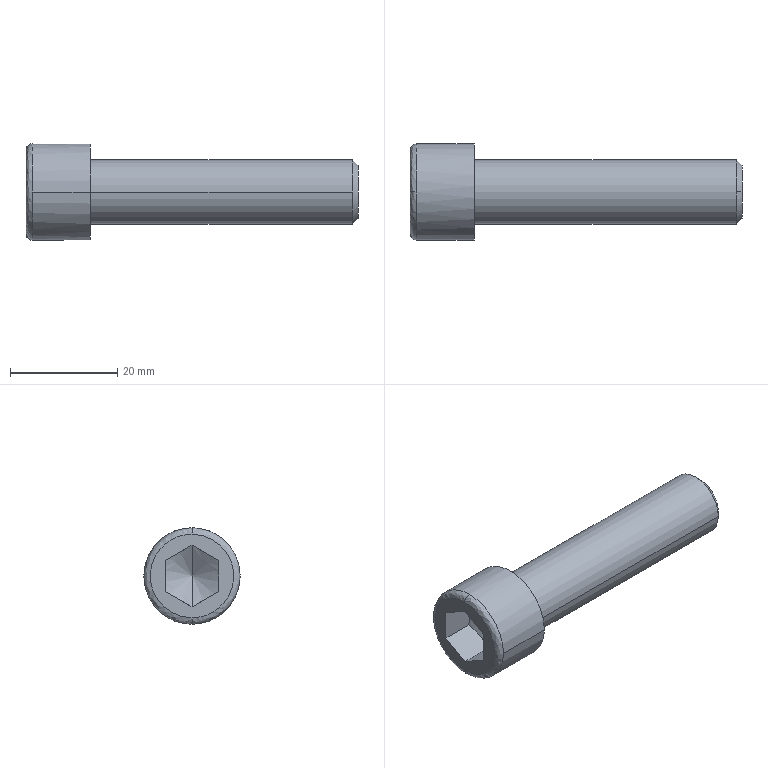Part | SolidWorks | features BaseBody 1 | 1 solid | 21 faces | box 62 x 18 x 18 mm | volume 8038 mm3 | plane 9 | spline 4 | cylinder 4 | cone 4 | commonest cylinder face diameters 12 x2 18 x2
STEP:
#1=CARTESIAN_POINT('',(0.,0.,6.1));
#2=VERTEX_POINT('',#1);
#3=CARTESIAN_POINT('',(0.,0.,-6.1));
#4=VERTEX_POINT('',#3);
#5=CARTESIAN_POINT('',(0.,0.,6.1));
#6=CARTESIAN_POINT('',(0.,0.1864,6.1));
#7=CARTESIAN_POINT('',(0.,0.4649,6.087));
#8=CARTESIAN_POINT('',(0.,0.788,6.05));
#9=CARTESIAN_POINT('',(0.,0.9492,6.026));
#10=CARTESIAN_POINT('',(0.,1.018,6.014));
#11=CARTESIAN_POINT('',(0.,1.064,6.007));
#12=CARTESIAN_POINT('',(0.,1.086,6.003));
#13=CARTESIAN_POINT('',(0.,1.304,5.962));
#14=CARTESIAN_POINT('',(0.,1.592,5.894));
#15=CARTESIAN_POINT('',(0.,1.921,5.791));
#16=CARTESIAN_POINT('',(0.,2.06,5.742));
#17=CARTESIAN_POINT('',(0.,2.153,5.708));
#18=CARTESIAN_POINT('',(0.,2.198,5.691));
#19=CARTESIAN_POINT('',(0.,2.437,5.596));
#20=CARTESIAN_POINT('',(0.,2.717,5.468));
#21=CARTESIAN_POINT('',(0.,2.987,5.32));
#22=CARTESIAN_POINT('',(0.,3.164,5.216));
#23=CARTESIAN_POINT('',(0.,3.25,5.163));
#24=CARTESIAN_POINT('',(0.,3.69,4.875));
#25=CARTESIAN_POINT('',(0.,4.016,4.611));
#26=CARTESIAN_POINT('',(0.,4.462,4.165));
#27=CARTESIAN_POINT('',(0.,4.673,3.931));
#28=CARTESIAN_POINT('',(0.,4.897,3.641));
#29=CARTESIAN_POINT('',(0.,4.988,3.512));
#30=CARTESIAN_POINT('',(0.,5.047,3.426));
#31=CARTESIAN_POINT('',(0.,5.077,3.381));
#32=CARTESIAN_POINT('',(0.,5.218,3.166));
#33=CARTESIAN_POINT('',(0.,5.374,2.9));
#34=CARTESIAN_POINT('',(0.,5.531,2.577));
#35=CARTESIAN_POINT('',(0.,5.593,2.436));
#36=CARTESIAN_POINT('',(0.,5.633,2.341));
#37=CARTESIAN_POINT('',(0.,5.654,2.291));
#38=CARTESIAN_POINT('',(0.,5.744,2.062));
#39=CARTESIAN_POINT('',(0.,5.84,1.782));
#40=CARTESIAN_POINT('',(0.,5.927,1.448));
#41=CARTESIAN_POINT('',(0.,5.965,1.28));
#42=CARTESIAN_POINT('',(0.,5.979,1.207));
#43=CARTESIAN_POINT('',(0.,5.989,1.159));
#44=CARTESIAN_POINT('',(0.,5.994,1.133));
#45=CARTESIAN_POINT('',(0.,6.066,0.7429));
#46=CARTESIAN_POINT('',(0.,6.1,0.3729));
#47=CARTESIAN_POINT('',(0.,6.1,-0.1865));
#48=CARTESIAN_POINT('',(0.,6.091,-0.3725));
#49=CARTESIAN_POINT('',(0.,6.066,-0.65));
#50=CARTESIAN_POINT('',(0.,6.05,-0.7884));
#51=CARTESIAN_POINT('',(0.,6.026,-0.9494));
#52=CARTESIAN_POINT('',(0.,6.014,-1.018));
#53=CARTESIAN_POINT('',(0.,6.007,-1.064));
#54=CARTESIAN_POINT('',(0.,6.003,-1.086));
#55=CARTESIAN_POINT('',(0.,5.962,-1.304));
#56=CARTESIAN_POINT('',(0.,5.894,-1.592));
#57=CARTESIAN_POINT('',(0.,5.791,-1.921));
#58=CARTESIAN_POINT('',(0.,5.742,-2.06));
#59=CARTESIAN_POINT('',(0.,5.708,-2.153));
#60=CARTESIAN_POINT('',(0.,5.691,-2.198));
#61=CARTESIAN_POINT('',(0.,5.596,-2.437));
#62=CARTESIAN_POINT('',(0.,5.468,-2.717));
#63=CARTESIAN_POINT('',(0.,5.32,-2.987));
#64=CARTESIAN_POINT('',(0.,5.216,-3.164));
#65=CARTESIAN_POINT('',(0.,5.163,-3.25));
#66=CARTESIAN_POINT('',(0.,4.875,-3.69));
#67=CARTESIAN_POINT('',(0.,4.611,-4.016));
#68=CARTESIAN_POINT('',(0.,4.165,-4.462));
#69=CARTESIAN_POINT('',(0.,3.931,-4.673));
#70=CARTESIAN_POINT('',(0.,3.641,-4.897));
#71=CARTESIAN_POINT('',(0.,3.512,-4.988));
#72=CARTESIAN_POINT('',(0.,3.426,-5.047));
#73=CARTESIAN_POINT('',(0.,3.381,-5.077));
#74=CARTESIAN_POINT('',(0.,3.166,-5.218));
#75=CARTESIAN_POINT('',(0.,2.9,-5.374));
#76=CARTESIAN_POINT('',(0.,2.577,-5.531));
#77=CARTESIAN_POINT('',(0.,2.436,-5.593));
#78=CARTESIAN_POINT('',(0.,2.341,-5.633));
#79=CARTESIAN_POINT('',(0.,2.291,-5.654));
#80=CARTESIAN_POINT('',(0.,2.062,-5.744));
#81=CARTESIAN_POINT('',(0.,1.782,-5.84));
#82=CARTESIAN_POINT('',(0.,1.448,-5.927));
#83=CARTESIAN_POINT('',(0.,1.28,-5.965));
#84=CARTESIAN_POINT('',(0.,1.207,-5.979));
#85=CARTESIAN_POINT('',(0.,1.159,-5.989));
#86=CARTESIAN_POINT('',(0.,1.133,-5.994));
#87=CARTESIAN_POINT('',(0.,0.7435,-6.066));
#88=CARTESIAN_POINT('',(0.,0.3728,-6.1));
#89=CARTESIAN_POINT('',(0.,0.,-6.1));
#90=B_SPLINE_CURVE_WITH_KNOTS('',3,(#5,#6,#7,#8,#9,#10,#11,#12,#13,#14,#15,#16,#17,#18,#19,#20,#21,#22,#23,#24,#25,#26,#27,#28,#29,#30,#31,#32,#33,#34,#35,#36,#37,#38,#39,#40,#41,#42,#43,#44,#45,#46,#47,#48,#49,#50,#51,#52,#53,#54,#55,#56,#57,#58,#59,#60,#61,#62,#63,#64,#65,#66,#67,#68,#69,#70,#71,#72,#73,#74,#75,#76,#77,#78,#79,#80,#81,#82,#83,#84,#85,#86,#87,#88,#89),.UNSPECIFIED.,.F.,.F.,(4,1,1,1,2,2,1,1,2,2,1,2,2,2,1,1,2,2,1,1,2,2,1,1,1,2,2,2,2,1,1,2,2,1,1,2,2,1,2,2,2,1,1,2,2,1,1,2,2,1,1,1,2,2,4),(0.75,0.7656,0.7734,0.7773,0.7793,0.7812,0.7969,0.8047,0.8086,0.8125,0.8281,0.8359,0.8437,0.875,0.8906,0.8984,0.9023,0.9063,0.9219,0.9297,0.9336,0.9375,0.9531,0.9609,0.9648,0.9668,0.9688,1.,1.016,1.023,1.027,1.029,1.031,1.047,1.055,1.059,1.063,1.078,1.086,1.094,1.125,1.141,1.148,1.152,1.156,1.172,1.18,1.184,1.188,1.203,1.211,1.215,1.217,1.219,1.25),.UNSPECIFIED.);
#91=EDGE_CURVE('',#2,#4,#90,.T.);
#92=ORIENTED_EDGE('',*,*,#91,.F.);
#93=CARTESIAN_POINT('',(0.1,0.,6.));
#94=VERTEX_POINT('',#93);
#95=CARTESIAN_POINT('',(0.1,0.,6.1));
#96=DIRECTION('',(0.,-1.,0.));
#97=DIRECTION('',(0.,0.,1.));
#98=AXIS2_PLACEMENT_3D('',#95,#96,#97);
#99=CIRCLE('',#98,0.1);
#100=EDGE_CURVE('',#2,#94,#99,.T.);
#101=ORIENTED_EDGE('',*,*,#100,.T.);
#102=CARTESIAN_POINT('',(0.1,6.,0.));
#103=VERTEX_POINT('',#102);
#104=CARTESIAN_POINT('',(0.1,0.,0.));
#105=DIRECTION('',(1.,0.,0.));
#106=DIRECTION('',(0.,1.,0.));
#107=AXIS2_PLACEMENT_3D('',#104,#105,#106);
#108=CIRCLE('',#107,6.);
#109=EDGE_CURVE('',#103,#94,#108,.T.);
#110=ORIENTED_EDGE('',*,*,#109,.F.);
#111=CARTESIAN_POINT('',(0.1,0.,-6.));
#112=VERTEX_POINT('',#111);
#113=CARTESIAN_POINT('',(0.1,0.,0.));
#114=DIRECTION('',(1.,0.,0.));
#115=DIRECTION('',(0.,1.,0.));
#116=AXIS2_PLACEMENT_3D('',#113,#114,#115);
#117=CIRCLE('',#116,6.);
#118=EDGE_CURVE('',#112,#103,#117,.T.);
#119=ORIENTED_EDGE('',*,*,#118,.F.);
#120=CARTESIAN_POINT('',(0.1,0.,-6.1));
#121=DIRECTION('',(0.,1.,0.));
#122=DIRECTION('',(0.,0.,-1.));
#123=AXIS2_PLACEMENT_3D('',#120,#121,#122);
#124=CIRCLE('',#123,0.1);
#125=EDGE_CURVE('',#4,#112,#124,.T.);
#126=ORIENTED_EDGE('',*,*,#125,.F.);
#127=EDGE_LOOP('',(#92,#101,#110,#119,#126));
#128=FACE_OUTER_BOUND('',#127,.T.);
#129=CARTESIAN_POINT('',(0.,0.,-6.1));
#130=CARTESIAN_POINT('',(0.,12.2,-6.1));
#131=CARTESIAN_POINT('',(0.,12.2,6.1));
#132=CARTESIAN_POINT('',(0.,0.,6.1));
#133=CARTESIAN_POINT('',(0.,0.,-6.041));
#134=CARTESIAN_POINT('',(0.,12.083,-6.041));
#135=CARTESIAN_POINT('',(0.,12.083,6.041));
#136=CARTESIAN_POINT('',(0.,0.,6.041));
#137=CARTESIAN_POINT('',(0.04142,0.,-6.));
#138=CARTESIAN_POINT('',(0.04142,12.,-6.));
#139=CARTESIAN_POINT('',(0.04142,12.,6.));
#140=CARTESIAN_POINT('',(0.04142,0.,6.));
#141=CARTESIAN_POINT('',(0.1,0.,-6.));
#142=CARTESIAN_POINT('',(0.1,12.,-6.));
#143=CARTESIAN_POINT('',(0.1,12.,6.));
#144=CARTESIAN_POINT('',(0.1,0.,6.));
#145=(BOUNDED_SURFACE()B_SPLINE_SURFACE(3,3,((#129,#130,#131,#132),(#133,#134,#135,#136),(#137,#138,#139,#140),(#141,#142,#143,#144)),.UNSPECIFIED.,.F.,.F.,.T.)B_SPLINE_SURFACE_WITH_KNOTS((4,4),(4,4),(0.,1.),(0.,1.),.UNSPECIFIED.)GEOMETRIC_REPRESENTATION_ITEM()RATIONAL_B_SPLINE_SURFACE(((1.,0.3333,0.3333,1.),(0.8047,0.2682,0.2682,0.8047),(0.8047,0.2682,0.2682,0.8047),(1.,0.3333,0.3333,1.)))REPRESENTATION_ITEM('')SURFACE());
#146=ADVANCED_FACE('',(#128),#145,.F.);
#147=CARTESIAN_POINT('',(-10.8,0.,9.));
#148=VERTEX_POINT('',#147);
#149=CARTESIAN_POINT('',(-10.8,-9.,0.));
#150=VERTEX_POINT('',#149);
#151=CARTESIAN_POINT('',(-10.8,0.,0.));
#152=DIRECTION('',(1.,0.,0.));
#153=DIRECTION('',(0.,1.,0.));
#154=AXIS2_PLACEMENT_3D('',#151,#152,#153);
#155=CIRCLE('',#154,9.);
#156=EDGE_CURVE('',#148,#150,#155,.T.);
#157=ORIENTED_EDGE('',*,*,#156,.F.);
#158=CARTESIAN_POINT('',(-12.,0.,7.8));
#159=VERTEX_POINT('',#158);
#160=CARTESIAN_POINT('',(-10.8,0.,7.8));
#161=DIRECTION('',(0.,-1.,0.));
#162=DIRECTION('',(0.,0.,1.));
#163=AXIS2_PLACEMENT_3D('',#160,#161,#162);
#164=CIRCLE('',#163,1.2);
#165=EDGE_CURVE('',#148,#159,#164,.T.);
#166=ORIENTED_EDGE('',*,*,#165,.T.);
#167=CARTESIAN_POINT('',(-12.,0.,-7.8));
#168=VERTEX_POINT('',#167);
#169=CARTESIAN_POINT('',(-12.,0.,7.8));
#170=CARTESIAN_POINT('',(-12.,-15.6,7.8));
#171=CARTESIAN_POINT('',(-12.,-15.6,-7.8));
#172=CARTESIAN_POINT('',(-12.,0.,-7.8));
#173=(BOUNDED_CURVE()B_SPLINE_CURVE(3,(#169,#170,#171,#172),.UNSPECIFIED.,.F.,.T.)B_SPLINE_CURVE_WITH_KNOTS((4,4),(0.25,0.75),.UNSPECIFIED.)CURVE()GEOMETRIC_REPRESENTATION_ITEM()RATIONAL_B_SPLINE_CURVE((1.,0.3333,0.3333,1.))REPRESENTATION_ITEM(''));
#174=EDGE_CURVE('',#159,#168,#173,.T.);
#175=ORIENTED_EDGE('',*,*,#174,.T.);
#176=CARTESIAN_POINT('',(-10.8,0.,-9.));
#177=VERTEX_POINT('',#176);
#178=CARTESIAN_POINT('',(-10.8,0.,-7.8));
#179=DIRECTION('',(0.,1.,0.));
#180=DIRECTION('',(0.,0.,-1.));
#181=AXIS2_PLACEMENT_3D('',#178,#179,#180);
#182=CIRCLE('',#181,1.2);
#183=EDGE_CURVE('',#177,#168,#182,.T.);
#184=ORIENTED_EDGE('',*,*,#183,.F.);
#185=CARTESIAN_POINT('',(-10.8,0.,0.));
#186=DIRECTION('',(1.,0.,0.));
#187=DIRECTION('',(0.,1.,0.));
#188=AXIS2_PLACEMENT_3D('',#185,#186,#187);
#189=CIRCLE('',#188,9.);
#190=EDGE_CURVE('',#150,#177,#189,.T.);
#191=ORIENTED_EDGE('',*,*,#190,.F.);
#192=EDGE_LOOP('',(#157,#166,#175,#184,#191));
#193=FACE_OUTER_BOUND('',#192,.T.);
#194=CARTESIAN_POINT('',(-10.8,0.,9.));
#195=CARTESIAN_POINT('',(-10.8,-18.,9.));
#196=CARTESIAN_POINT('',(-10.8,-18.,-9.));
#197=CARTESIAN_POINT('',(-10.8,0.,-9.));
#198=CARTESIAN_POINT('',(-11.503,0.,9.));
#199=CARTESIAN_POINT('',(-11.503,-18.,9.));
#200=CARTESIAN_POINT('',(-11.503,-18.,-9.));
#201=CARTESIAN_POINT('',(-11.503,0.,-9.));
#202=CARTESIAN_POINT('',(-12.,0.,8.503));
#203=CARTESIAN_POINT('',(-12.,-17.006,8.503));
#204=CARTESIAN_POINT('',(-12.,-17.006,-8.503));
#205=CARTESIAN_POINT('',(-12.,0.,-8.503));
#206=CARTESIAN_POINT('',(-12.,0.,7.8));
#207=CARTESIAN_POINT('',(-12.,-15.6,7.8));
#208=CARTESIAN_POINT('',(-12.,-15.6,-7.8));
#209=CARTESIAN_POINT('',(-12.,0.,-7.8));
#210=(BOUNDED_SURFACE()B_SPLINE_SURFACE(3,3,((#194,#195,#196,#197),(#198,#199,#200,#201),(#202,#203,#204,#205),(#206,#207,#208,#209)),.UNSPECIFIED.,.F.,.F.,.T.)B_SPLINE_SURFACE_WITH_KNOTS((4,4),(4,4),(0.,1.),(0.,1.),.UNSPECIFIED.)GEOMETRIC_REPRESENTATION_ITEM()RATIONAL_B_SPLINE_SURFACE(((1.,0.3333,0.3333,1.),(0.8047,0.2682,0.2682,0.8047),(0.8047,0.2682,0.2682,0.8047),(1.,0.3333,0.3333,1.)))REPRESENTATION_ITEM('')SURFACE());
#211=ADVANCED_FACE('',(#193),#210,.T.);
#212=ORIENTED_EDGE('',*,*,#109,.T.);
#213=CARTESIAN_POINT('',(0.1,-6.,0.));
#214=VERTEX_POINT('',#213);
#215=CARTESIAN_POINT('',(0.1,0.,0.));
#216=DIRECTION('',(1.,0.,0.));
#217=DIRECTION('',(0.,1.,0.));
#218=AXIS2_PLACEMENT_3D('',#215,#216,#217);
#219=CIRCLE('',#218,6.);
#220=EDGE_CURVE('',#94,#214,#219,.T.);
#221=ORIENTED_EDGE('',*,*,#220,.T.);
#222=CARTESIAN_POINT('',(48.926,-6.,0.));
#223=VERTEX_POINT('',#222);
#224=CARTESIAN_POINT('',(35.,-6.,0.));
#225=DIRECTION('',(1.,0.,0.));
#226=VECTOR('',#225,1000.);
#227=LINE('',#224,#226);
#228=EDGE_CURVE('',#214,#223,#227,.T.);
#229=ORIENTED_EDGE('',*,*,#228,.T.);
#230=CARTESIAN_POINT('',(48.926,0.,6.));
#231=VERTEX_POINT('',#230);
#232=CARTESIAN_POINT('',(48.926,0.,0.));
#233=DIRECTION('',(-1.,0.,0.));
#234=DIRECTION('',(0.,1.,0.));
#235=AXIS2_PLACEMENT_3D('',#232,#233,#234);
#236=CIRCLE('',#235,6.);
#237=EDGE_CURVE('',#223,#231,#236,.T.);
#238=ORIENTED_EDGE('',*,*,#237,.T.);
#239=CARTESIAN_POINT('',(48.926,6.,0.));
#240=VERTEX_POINT('',#239);
#241=CARTESIAN_POINT('',(48.926,0.,0.));
#242=DIRECTION('',(-1.,0.,0.));
#243=DIRECTION('',(0.,1.,0.));
#244=AXIS2_PLACEMENT_3D('',#241,#242,#243);
#245=CIRCLE('',#244,6.);
#246=EDGE_CURVE('',#231,#240,#245,.T.);
#247=ORIENTED_EDGE('',*,*,#246,.T.);
#248=CARTESIAN_POINT('',(35.,6.,0.));
#249=DIRECTION('',(1.,0.,0.));
#250=VECTOR('',#249,1000.);
#251=LINE('',#248,#250);
#252=EDGE_CURVE('',#103,#240,#251,.T.);
#253=ORIENTED_EDGE('',*,*,#252,.F.);
#254=EDGE_LOOP('',(#212,#221,#229,#238,#247,#253));
#255=FACE_OUTER_BOUND('',#254,.T.);
#256=CARTESIAN_POINT('',(35.,0.,0.));
#257=DIRECTION('',(1.,0.,0.));
#258=DIRECTION('',(0.,1.,0.));
#259=AXIS2_PLACEMENT_3D('',#256,#257,#258);
#260=CYLINDRICAL_SURFACE('',#259,6.);
#261=ADVANCED_FACE('',(#255),#260,.T.);
#262=CARTESIAN_POINT('',(50.,0.,4.926));
#263=VERTEX_POINT('',#262);
#264=CARTESIAN_POINT('',(50.,0.,-4.926));
#265=VERTEX_POINT('',#264);
#266=CARTESIAN_POINT('',(50.,0.,0.));
#267=DIRECTION('',(-1.,0.,0.));
#268=DIRECTION('',(0.,0.,1.));
#269=AXIS2_PLACEMENT_3D('',#266,#267,#268);
#270=CIRCLE('',#269,4.926);
#271=EDGE_CURVE('',#263,#265,#270,.T.);
#272=ORIENTED_EDGE('',*,*,#271,.T.);
#273=CARTESIAN_POINT('',(48.926,0.,-6.));
#274=VERTEX_POINT('',#273);
#275=CARTESIAN_POINT('',(48.926,0.,-6.));
#276=DIRECTION('',(-0.7071,0.,-0.7071));
#277=VECTOR('',#276,1000.);
#278=LINE('',#275,#277);
#279=EDGE_CURVE('',#265,#274,#278,.T.);
#280=ORIENTED_EDGE('',*,*,#279,.T.);
#281=CARTESIAN_POINT('',(48.926,0.,0.));
#282=DIRECTION('',(-1.,0.,0.));
#283=DIRECTION('',(0.,1.,0.));
#284=AXIS2_PLACEMENT_3D('',#281,#282,#283);
#285=CIRCLE('',#284,6.);
#286=EDGE_CURVE('',#240,#274,#285,.T.);
#287=ORIENTED_EDGE('',*,*,#286,.F.);
#288=ORIENTED_EDGE('',*,*,#246,.F.);
#289=CARTESIAN_POINT('',(48.926,0.,6.));
#290=DIRECTION('',(-0.7071,0.,0.7071));
#291=VECTOR('',#290,1000.);
#292=LINE('',#289,#291);
#293=EDGE_CURVE('',#263,#231,#292,.T.);
#294=ORIENTED_EDGE('',*,*,#293,.F.);
#295=EDGE_LOOP('',(#272,#280,#287,#288,#294));
#296=FACE_OUTER_BOUND('',#295,.T.);
#297=CARTESIAN_POINT('',(48.926,0.,0.));
#298=DIRECTION('',(-1.,0.,0.));
#299=DIRECTION('',(0.,0.,1.));
#300=AXIS2_PLACEMENT_3D('',#297,#298,#299);
#301=CONICAL_SURFACE('',#300,6.,0.7854);
#302=ADVANCED_FACE('',(#296),#301,.T.);
#303=CARTESIAN_POINT('',(-10.8,9.,0.));
#304=VERTEX_POINT('',#303);
#305=CARTESIAN_POINT('',(-10.8,0.,0.));
#306=DIRECTION('',(1.,0.,0.));
#307=DIRECTION('',(0.,1.,0.));
#308=AXIS2_PLACEMENT_3D('',#305,#306,#307);
#309=CIRCLE('',#308,9.);
#310=EDGE_CURVE('',#304,#148,#309,.T.);
#311=ORIENTED_EDGE('',*,*,#310,.T.);
#312=ORIENTED_EDGE('',*,*,#156,.T.);
#313=CARTESIAN_POINT('',(0.,-9.,0.));
#314=VERTEX_POINT('',#313);
#315=CARTESIAN_POINT('',(-6.,-9.,0.));
#316=DIRECTION('',(1.,0.,0.));
#317=VECTOR('',#316,1000.);
#318=LINE('',#315,#317);
#319=EDGE_CURVE('',#150,#314,#318,.T.);
#320=ORIENTED_EDGE('',*,*,#319,.T.);
#321=CARTESIAN_POINT('',(0.,9.,0.));
#322=VERTEX_POINT('',#321);
#323=CARTESIAN_POINT('',(0.,0.,0.));
#324=DIRECTION('',(1.,0.,0.));
#325=DIRECTION('',(0.,1.,0.));
#326=AXIS2_PLACEMENT_3D('',#323,#324,#325);
#327=CIRCLE('',#326,9.);
#328=EDGE_CURVE('',#322,#314,#327,.T.);
#329=ORIENTED_EDGE('',*,*,#328,.F.);
#330=CARTESIAN_POINT('',(-6.,9.,0.));
#331=DIRECTION('',(1.,0.,0.));
#332=VECTOR('',#331,1000.);
#333=LINE('',#330,#332);
#334=EDGE_CURVE('',#304,#322,#333,.T.);
#335=ORIENTED_EDGE('',*,*,#334,.F.);
#336=EDGE_LOOP('',(#311,#312,#320,#329,#335));
#337=FACE_OUTER_BOUND('',#336,.T.);
#338=CARTESIAN_POINT('',(-6.,0.,0.));
#339=DIRECTION('',(1.,0.,0.));
#340=DIRECTION('',(0.,1.,0.));
#341=AXIS2_PLACEMENT_3D('',#338,#339,#340);
#342=CYLINDRICAL_SURFACE('',#341,9.);
#343=ADVANCED_FACE('',(#337),#342,.T.);
#344=CARTESIAN_POINT('',(-2.667,0.,0.));
#345=VERTEX_POINT('',#344);
#346=CARTESIAN_POINT('',(-6.,0.,5.774));
#347=VERTEX_POINT('',#346);
#348=CARTESIAN_POINT('',(-6.02,0.,5.808));
#349=DIRECTION('',(-0.5,0.,0.866));
#350=VECTOR('',#349,1000.);
#351=LINE('',#348,#350);
#352=EDGE_CURVE('',#345,#347,#351,.T.);
#353=ORIENTED_EDGE('',*,*,#352,.F.);
#354=CARTESIAN_POINT('',(-6.,0.,-5.774));
#355=VERTEX_POINT('',#354);
#356=CARTESIAN_POINT('',(-6.02,0.,-5.808));
#357=DIRECTION('',(-0.5,0.,-0.866));
#358=VECTOR('',#357,1000.);
#359=LINE('',#356,#358);
#360=EDGE_CURVE('',#345,#355,#359,.T.);
#361=ORIENTED_EDGE('',*,*,#360,.T.);
#362=CARTESIAN_POINT('',(-6.,-5.,-2.887));
#363=VERTEX_POINT('',#362);
#364=CARTESIAN_POINT('',(-6.,0.,-5.774));
#365=CARTESIAN_POINT('',(-5.728,-0.8164,-5.302));
#366=CARTESIAN_POINT('',(-5.554,-1.645,-4.824));
#367=CARTESIAN_POINT('',(-5.553,-2.708,-4.21));
#368=CARTESIAN_POINT('',(-5.564,-2.921,-4.087));
#369=CARTESIAN_POINT('',(-5.604,-3.344,-3.843));
#370=CARTESIAN_POINT('',(-5.635,-3.554,-3.722));
#371=CARTESIAN_POINT('',(-5.751,-4.179,-3.361));
#372=CARTESIAN_POINT('',(-5.864,-4.591,-3.123));
#373=CARTESIAN_POINT('',(-6.,-5.,-2.887));
#374=B_SPLINE_CURVE_WITH_KNOTS('',3,(#364,#365,#366,#367,#368,#369,#370,#371,#372,#373),.UNSPECIFIED.,.F.,.F.,(4,2,2,2,4),(0.,0.002915,0.003644,0.004373,0.005831),.UNSPECIFIED.);
#375=EDGE_CURVE('',#355,#363,#374,.T.);
#376=ORIENTED_EDGE('',*,*,#375,.T.);
#377=CARTESIAN_POINT('',(-6.,-5.,2.887));
#378=VERTEX_POINT('',#377);
#379=CARTESIAN_POINT('',(-6.,-5.,-2.887));
#380=CARTESIAN_POINT('',(-5.728,-5.,-1.944));
#381=CARTESIAN_POINT('',(-5.554,-5.,-0.9872));
#382=CARTESIAN_POINT('',(-5.553,-5.,0.2399));
#383=CARTESIAN_POINT('',(-5.564,-5.,0.4865));
#384=CARTESIAN_POINT('',(-5.604,-5.,0.9743));
#385=CARTESIAN_POINT('',(-5.635,-5.,1.216));
#386=CARTESIAN_POINT('',(-5.751,-5.,1.939));
#387=CARTESIAN_POINT('',(-5.864,-5.,2.415));
#388=CARTESIAN_POINT('',(-6.,-5.,2.887));
#389=B_SPLINE_CURVE_WITH_KNOTS('',3,(#379,#380,#381,#382,#383,#384,#385,#386,#387,#388),.UNSPECIFIED.,.F.,.F.,(4,2,2,2,4),(0.,0.002915,0.003644,0.004373,0.005831),.UNSPECIFIED.);
#390=EDGE_CURVE('',#363,#378,#389,.T.);
#391=ORIENTED_EDGE('',*,*,#390,.T.);
#392=CARTESIAN_POINT('',(-6.,-5.,2.887));
#393=CARTESIAN_POINT('',(-5.728,-4.184,3.358));
#394=CARTESIAN_POINT('',(-5.554,-3.355,3.837));
#395=CARTESIAN_POINT('',(-5.553,-2.292,4.45));
#396=CARTESIAN_POINT('',(-5.564,-2.079,4.573));
#397=CARTESIAN_POINT('',(-5.604,-1.656,4.817));
#398=CARTESIAN_POINT('',(-5.635,-1.446,4.938));
#399=CARTESIAN_POINT('',(-5.751,-0.8208,5.3));
#400=CARTESIAN_POINT('',(-5.864,-0.4087,5.538));
#401=CARTESIAN_POINT('',(-6.,0.,5.774));
#402=B_SPLINE_CURVE_WITH_KNOTS('',3,(#392,#393,#394,#395,#396,#397,#398,#399,#400,#401),.UNSPECIFIED.,.F.,.F.,(4,2,2,2,4),(0.,0.002915,0.003644,0.004373,0.005831),.UNSPECIFIED.);
#403=EDGE_CURVE('',#378,#347,#402,.T.);
#404=ORIENTED_EDGE('',*,*,#403,.T.);
#405=EDGE_LOOP('',(#353,#361,#376,#391,#404));
#406=FACE_OUTER_BOUND('',#405,.T.);
#407=CARTESIAN_POINT('',(-6.02,0.,0.));
#408=DIRECTION('',(-1.,0.,0.));
#409=DIRECTION('',(0.,0.,1.));
#410=AXIS2_PLACEMENT_3D('',#407,#408,#409);
#411=CONICAL_SURFACE('',#410,5.808,1.047);
#412=ADVANCED_FACE('',(#406),#411,.F.);
#413=ORIENTED_EDGE('',*,*,#228,.F.);
#414=CARTESIAN_POINT('',(0.1,0.,0.));
#415=DIRECTION('',(1.,0.,0.));
#416=DIRECTION('',(0.,1.,0.));
#417=AXIS2_PLACEMENT_3D('',#414,#415,#416);
#418=CIRCLE('',#417,6.);
#419=EDGE_CURVE('',#214,#112,#418,.T.);
#420=ORIENTED_EDGE('',*,*,#419,.T.);
#421=ORIENTED_EDGE('',*,*,#118,.T.);
#422=ORIENTED_EDGE('',*,*,#252,.T.);
#423=ORIENTED_EDGE('',*,*,#286,.T.);
#424=CARTESIAN_POINT('',(48.926,0.,0.));
#425=DIRECTION('',(-1.,0.,0.));
#426=DIRECTION('',(0.,1.,0.));
#427=AXIS2_PLACEMENT_3D('',#424,#425,#426);
#428=CIRCLE('',#427,6.);
#429=EDGE_CURVE('',#274,#223,#428,.T.);
#430=ORIENTED_EDGE('',*,*,#429,.T.);
#431=EDGE_LOOP('',(#413,#420,#421,#422,#423,#430));
#432=FACE_OUTER_BOUND('',#431,.T.);
#433=CARTESIAN_POINT('',(35.,0.,0.));
#434=DIRECTION('',(1.,0.,0.));
#435=DIRECTION('',(0.,1.,0.));
#436=AXIS2_PLACEMENT_3D('',#433,#434,#435);
#437=CYLINDRICAL_SURFACE('',#436,6.);
#438=ADVANCED_FACE('',(#432),#437,.T.);
#439=ORIENTED_EDGE('',*,*,#100,.F.);
#440=CARTESIAN_POINT('',(0.,0.,-6.1));
#441=CARTESIAN_POINT('',(0.,-0.1864,-6.1));
#442=CARTESIAN_POINT('',(0.,-0.4649,-6.087));
#443=CARTESIAN_POINT('',(0.,-0.788,-6.05));
#444=CARTESIAN_POINT('',(0.,-0.9492,-6.026));
#445=CARTESIAN_POINT('',(0.,-1.018,-6.014));
#446=CARTESIAN_POINT('',(0.,-1.064,-6.007));
#447=CARTESIAN_POINT('',(0.,-1.086,-6.003));
#448=CARTESIAN_POINT('',(0.,-1.304,-5.962));
#449=CARTESIAN_POINT('',(0.,-1.592,-5.894));
#450=CARTESIAN_POINT('',(0.,-1.921,-5.791));
#451=CARTESIAN_POINT('',(0.,-2.06,-5.742));
#452=CARTESIAN_POINT('',(0.,-2.153,-5.708));
#453=CARTESIAN_POINT('',(0.,-2.198,-5.691));
#454=CARTESIAN_POINT('',(0.,-2.437,-5.596));
#455=CARTESIAN_POINT('',(0.,-2.717,-5.468));
#456=CARTESIAN_POINT('',(0.,-2.987,-5.32));
#457=CARTESIAN_POINT('',(0.,-3.164,-5.216));
#458=CARTESIAN_POINT('',(0.,-3.25,-5.163));
#459=CARTESIAN_POINT('',(0.,-3.69,-4.875));
#460=CARTESIAN_POINT('',(0.,-4.016,-4.611));
#461=CARTESIAN_POINT('',(0.,-4.462,-4.165));
#462=CARTESIAN_POINT('',(0.,-4.673,-3.931));
#463=CARTESIAN_POINT('',(0.,-4.897,-3.641));
#464=CARTESIAN_POINT('',(0.,-4.988,-3.512));
#465=CARTESIAN_POINT('',(0.,-5.047,-3.426));
#466=CARTESIAN_POINT('',(0.,-5.077,-3.381));
#467=CARTESIAN_POINT('',(0.,-5.218,-3.166));
#468=CARTESIAN_POINT('',(0.,-5.374,-2.9));
#469=CARTESIAN_POINT('',(0.,-5.531,-2.577));
#470=CARTESIAN_POINT('',(0.,-5.593,-2.436));
#471=CARTESIAN_POINT('',(0.,-5.633,-2.341));
#472=CARTESIAN_POINT('',(0.,-5.654,-2.291));
#473=CARTESIAN_POINT('',(0.,-5.744,-2.062));
#474=CARTESIAN_POINT('',(0.,-5.84,-1.782));
#475=CARTESIAN_POINT('',(0.,-5.927,-1.448));
#476=CARTESIAN_POINT('',(0.,-5.965,-1.28));
#477=CARTESIAN_POINT('',(0.,-5.979,-1.207));
#478=CARTESIAN_POINT('',(0.,-5.989,-1.159));
#479=CARTESIAN_POINT('',(0.,-5.994,-1.133));
#480=CARTESIAN_POINT('',(0.,-6.066,-0.7435));
#481=CARTESIAN_POINT('',(0.,-6.1,-0.3728));
#482=CARTESIAN_POINT('',(0.,-6.1,0.1864));
#483=CARTESIAN_POINT('',(0.,-6.087,0.4649));
#484=CARTESIAN_POINT('',(0.,-6.05,0.788));
#485=CARTESIAN_POINT('',(0.,-6.026,0.9492));
#486=CARTESIAN_POINT('',(0.,-6.014,1.018));
#487=CARTESIAN_POINT('',(0.,-6.007,1.064));
#488=CARTESIAN_POINT('',(0.,-6.003,1.086));
#489=CARTESIAN_POINT('',(0.,-5.962,1.304));
#490=CARTESIAN_POINT('',(0.,-5.894,1.592));
#491=CARTESIAN_POINT('',(0.,-5.791,1.921));
#492=CARTESIAN_POINT('',(0.,-5.742,2.06));
#493=CARTESIAN_POINT('',(0.,-5.708,2.153));
#494=CARTESIAN_POINT('',(0.,-5.691,2.198));
#495=CARTESIAN_POINT('',(0.,-5.596,2.437));
#496=CARTESIAN_POINT('',(0.,-5.468,2.717));
#497=CARTESIAN_POINT('',(0.,-5.32,2.987));
#498=CARTESIAN_POINT('',(0.,-5.216,3.164));
#499=CARTESIAN_POINT('',(0.,-5.163,3.25));
#500=CARTESIAN_POINT('',(0.,-4.875,3.69));
#501=CARTESIAN_POINT('',(0.,-4.611,4.016));
#502=CARTESIAN_POINT('',(0.,-4.165,4.462));
#503=CARTESIAN_POINT('',(0.,-3.931,4.673));
#504=CARTESIAN_POINT('',(0.,-3.641,4.897));
#505=CARTESIAN_POINT('',(0.,-3.512,4.988));
#506=CARTESIAN_POINT('',(0.,-3.426,5.047));
#507=CARTESIAN_POINT('',(0.,-3.381,5.077));
#508=CARTESIAN_POINT('',(0.,-3.166,5.218));
#509=CARTESIAN_POINT('',(0.,-2.9,5.374));
#510=CARTESIAN_POINT('',(0.,-2.577,5.531));
#511=CARTESIAN_POINT('',(0.,-2.436,5.593));
#512=CARTESIAN_POINT('',(0.,-2.341,5.633));
#513=CARTESIAN_POINT('',(0.,-2.291,5.654));
#514=CARTESIAN_POINT('',(0.,-2.062,5.744));
#515=CARTESIAN_POINT('',(0.,-1.782,5.84));
#516=CARTESIAN_POINT('',(0.,-1.448,5.927));
#517=CARTESIAN_POINT('',(0.,-1.28,5.965));
#518=CARTESIAN_POINT('',(0.,-1.207,5.979));
#519=CARTESIAN_POINT('',(0.,-1.159,5.989));
#520=CARTESIAN_POINT('',(0.,-1.133,5.994));
#521=CARTESIAN_POINT('',(0.,-0.7435,6.066));
#522=CARTESIAN_POINT('',(0.,-0.3728,6.1));
#523=CARTESIAN_POINT('',(0.,0.,6.1));
#524=B_SPLINE_CURVE_WITH_KNOTS('',3,(#440,#441,#442,#443,#444,#445,#446,#447,#448,#449,#450,#451,#452,#453,#454,#455,#456,#457,#458,#459,#460,#461,#462,#463,#464,#465,#466,#467,#468,#469,#470,#471,#472,#473,#474,#475,#476,#477,#478,#479,#480,#481,#482,#483,#484,#485,#486,#487,#488,#489,#490,#491,#492,#493,#494,#495,#496,#497,#498,#499,#500,#501,#502,#503,#504,#505,#506,#507,#508,#509,#510,#511,#512,#513,#514,#515,#516,#517,#518,#519,#520,#521,#522,#523),.UNSPECIFIED.,.F.,.F.,(4,1,1,1,2,2,1,1,2,2,1,2,2,2,1,1,2,2,1,1,2,2,1,1,1,2,2,2,1,1,1,2,2,1,1,2,2,1,2,2,2,1,1,2,2,1,1,2,2,1,1,1,2,2,4),(0.25,0.2656,0.2734,0.2773,0.2793,0.2813,0.2969,0.3047,0.3086,0.3125,0.3281,0.3359,0.3437,0.375,0.3906,0.3984,0.4023,0.4062,0.4219,0.4297,0.4336,0.4375,0.4531,0.4609,0.4648,0.4668,0.4687,0.5,0.5156,0.5234,0.5273,0.5293,0.5312,0.5469,0.5547,0.5586,0.5625,0.5781,0.5859,0.5937,0.625,0.6406,0.6484,0.6523,0.6562,0.6719,0.6797,0.6836,0.6875,0.7031,0.7109,0.7148,0.7168,0.7187,0.75),.UNSPECIFIED.);
#525=EDGE_CURVE('',#4,#2,#524,.T.);
#526=ORIENTED_EDGE('',*,*,#525,.F.);
#527=ORIENTED_EDGE('',*,*,#125,.T.);
#528=ORIENTED_EDGE('',*,*,#419,.F.);
#529=ORIENTED_EDGE('',*,*,#220,.F.);
#530=EDGE_LOOP('',(#439,#526,#527,#528,#529));
#531=FACE_OUTER_BOUND('',#530,.T.);
#532=CARTESIAN_POINT('',(0.,0.,6.1));
#533=CARTESIAN_POINT('',(0.,-12.2,6.1));
#534=CARTESIAN_POINT('',(0.,-12.2,-6.1));
#535=CARTESIAN_POINT('',(0.,0.,-6.1));
#536=CARTESIAN_POINT('',(0.,0.,6.041));
#537=CARTESIAN_POINT('',(0.,-12.083,6.041));
#538=CARTESIAN_POINT('',(0.,-12.083,-6.041));
#539=CARTESIAN_POINT('',(0.,0.,-6.041));
#540=CARTESIAN_POINT('',(0.04142,0.,6.));
#541=CARTESIAN_POINT('',(0.04142,-12.,6.));
#542=CARTESIAN_POINT('',(0.04142,-12.,-6.));
#543=CARTESIAN_POINT('',(0.04142,0.,-6.));
#544=CARTESIAN_POINT('',(0.1,0.,6.));
#545=CARTESIAN_POINT('',(0.1,-12.,6.));
#546=CARTESIAN_POINT('',(0.1,-12.,-6.));
#547=CARTESIAN_POINT('',(0.1,0.,-6.));
#548=(BOUNDED_SURFACE()B_SPLINE_SURFACE(3,3,((#532,#533,#534,#535),(#536,#537,#538,#539),(#540,#541,#542,#543),(#544,#545,#546,#547)),.UNSPECIFIED.,.F.,.F.,.T.)B_SPLINE_SURFACE_WITH_KNOTS((4,4),(4,4),(0.,1.),(0.,1.),.UNSPECIFIED.)GEOMETRIC_REPRESENTATION_ITEM()RATIONAL_B_SPLINE_SURFACE(((1.,0.3333,0.3333,1.),(0.8047,0.2682,0.2682,0.8047),(0.8047,0.2682,0.2682,0.8047),(1.,0.3333,0.3333,1.)))REPRESENTATION_ITEM('')SURFACE());
#549=ADVANCED_FACE('',(#531),#548,.F.);
#550=ORIENTED_EDGE('',*,*,#279,.F.);
#551=CARTESIAN_POINT('',(50.,0.,0.));
#552=DIRECTION('',(-1.,0.,0.));
#553=DIRECTION('',(0.,0.,1.));
#554=AXIS2_PLACEMENT_3D('',#551,#552,#553);
#555=CIRCLE('',#554,4.926);
#556=EDGE_CURVE('',#265,#263,#555,.T.);
#557=ORIENTED_EDGE('',*,*,#556,.T.);
#558=ORIENTED_EDGE('',*,*,#293,.T.);
#559=ORIENTED_EDGE('',*,*,#237,.F.);
#560=ORIENTED_EDGE('',*,*,#429,.F.);
#561=EDGE_LOOP('',(#550,#557,#558,#559,#560));
#562=FACE_OUTER_BOUND('',#561,.T.);
#563=CARTESIAN_POINT('',(48.926,0.,0.));
#564=DIRECTION('',(-1.,0.,0.));
#565=DIRECTION('',(0.,0.,1.));
#566=AXIS2_PLACEMENT_3D('',#563,#564,#565);
#567=CONICAL_SURFACE('',#566,6.,0.7854);
#568=ADVANCED_FACE('',(#562),#567,.T.);
#569=ORIENTED_EDGE('',*,*,#525,.T.);
#570=ORIENTED_EDGE('',*,*,#91,.T.);
#571=EDGE_LOOP('',(#569,#570));
#572=FACE_BOUND('',#571,.T.);
#573=ORIENTED_EDGE('',*,*,#328,.T.);
#574=CARTESIAN_POINT('',(0.,0.,0.));
#575=DIRECTION('',(1.,0.,0.));
#576=DIRECTION('',(0.,1.,0.));
#577=AXIS2_PLACEMENT_3D('',#574,#575,#576);
#578=CIRCLE('',#577,9.);
#579=EDGE_CURVE('',#314,#322,#578,.T.);
#580=ORIENTED_EDGE('',*,*,#579,.T.);
#581=EDGE_LOOP('',(#573,#580));
#582=FACE_OUTER_BOUND('',#581,.T.);
#583=CARTESIAN_POINT('',(0.,7.5,0.));
#584=DIRECTION('',(1.,0.,0.));
#585=DIRECTION('',(0.,1.,0.));
#586=AXIS2_PLACEMENT_3D('',#583,#584,#585);
#587=PLANE('',#586);
#588=ADVANCED_FACE('',(#572,#582),#587,.T.);
#589=ORIENTED_EDGE('',*,*,#271,.F.);
#590=ORIENTED_EDGE('',*,*,#556,.F.);
#591=EDGE_LOOP('',(#589,#590));
#592=FACE_OUTER_BOUND('',#591,.T.);
#593=CARTESIAN_POINT('',(50.,3.,0.));
#594=DIRECTION('',(1.,0.,0.));
#595=DIRECTION('',(0.,1.,0.));
#596=AXIS2_PLACEMENT_3D('',#593,#594,#595);
#597=PLANE('',#596);
#598=ADVANCED_FACE('',(#592),#597,.T.);
#599=ORIENTED_EDGE('',*,*,#319,.F.);
#600=ORIENTED_EDGE('',*,*,#190,.T.);
#601=CARTESIAN_POINT('',(-10.8,0.,0.));
#602=DIRECTION('',(1.,0.,0.));
#603=DIRECTION('',(0.,1.,0.));
#604=AXIS2_PLACEMENT_3D('',#601,#602,#603);
#605=CIRCLE('',#604,9.);
#606=EDGE_CURVE('',#177,#304,#605,.T.);
#607=ORIENTED_EDGE('',*,*,#606,.T.);
#608=ORIENTED_EDGE('',*,*,#334,.T.);
#609=ORIENTED_EDGE('',*,*,#579,.F.);
#610=EDGE_LOOP('',(#599,#600,#607,#608,#609));
#611=FACE_OUTER_BOUND('',#610,.T.);
#612=CARTESIAN_POINT('',(-6.,0.,0.));
#613=DIRECTION('',(1.,0.,0.));
#614=DIRECTION('',(0.,1.,0.));
#615=AXIS2_PLACEMENT_3D('',#612,#613,#614);
#616=CYLINDRICAL_SURFACE('',#615,9.);
#617=ADVANCED_FACE('',(#611),#616,.T.);
#618=ORIENTED_EDGE('',*,*,#165,.F.);
#619=ORIENTED_EDGE('',*,*,#310,.F.);
#620=ORIENTED_EDGE('',*,*,#606,.F.);
#621=ORIENTED_EDGE('',*,*,#183,.T.);
#622=CARTESIAN_POINT('',(-12.,0.,-7.8));
#623=CARTESIAN_POINT('',(-12.,15.6,-7.8));
#624=CARTESIAN_POINT('',(-12.,15.6,7.8));
#625=CARTESIAN_POINT('',(-12.,0.,7.8));
#626=(BOUNDED_CURVE()B_SPLINE_CURVE(3,(#622,#623,#624,#625),.UNSPECIFIED.,.F.,.F.)B_SPLINE_CURVE_WITH_KNOTS((4,4),(0.75,1.25),.UNSPECIFIED.)CURVE()GEOMETRIC_REPRESENTATION_ITEM()RATIONAL_B_SPLINE_CURVE((1.,0.3333,0.3333,1.))REPRESENTATION_ITEM(''));
#627=EDGE_CURVE('',#168,#159,#626,.T.);
#628=ORIENTED_EDGE('',*,*,#627,.T.);
#629=EDGE_LOOP('',(#618,#619,#620,#621,#628));
#630=FACE_OUTER_BOUND('',#629,.T.);
#631=CARTESIAN_POINT('',(-10.8,0.,-9.));
#632=CARTESIAN_POINT('',(-10.8,18.,-9.));
#633=CARTESIAN_POINT('',(-10.8,18.,9.));
#634=CARTESIAN_POINT('',(-10.8,0.,9.));
#635=CARTESIAN_POINT('',(-11.503,0.,-9.));
#636=CARTESIAN_POINT('',(-11.503,18.,-9.));
#637=CARTESIAN_POINT('',(-11.503,18.,9.));
#638=CARTESIAN_POINT('',(-11.503,0.,9.));
#639=CARTESIAN_POINT('',(-12.,0.,-8.503));
#640=CARTESIAN_POINT('',(-12.,17.006,-8.503));
#641=CARTESIAN_POINT('',(-12.,17.006,8.503));
#642=CARTESIAN_POINT('',(-12.,0.,8.503));
#643=CARTESIAN_POINT('',(-12.,0.,-7.8));
#644=CARTESIAN_POINT('',(-12.,15.6,-7.8));
#645=CARTESIAN_POINT('',(-12.,15.6,7.8));
#646=CARTESIAN_POINT('',(-12.,0.,7.8));
#647=(BOUNDED_SURFACE()B_SPLINE_SURFACE(3,3,((#631,#632,#633,#634),(#635,#636,#637,#638),(#639,#640,#641,#642),(#643,#644,#645,#646)),.UNSPECIFIED.,.F.,.F.,.T.)B_SPLINE_SURFACE_WITH_KNOTS((4,4),(4,4),(0.,1.),(0.,1.),.UNSPECIFIED.)GEOMETRIC_REPRESENTATION_ITEM()RATIONAL_B_SPLINE_SURFACE(((1.,0.3333,0.3333,1.),(0.8047,0.2682,0.2682,0.8047),(0.8047,0.2682,0.2682,0.8047),(1.,0.3333,0.3333,1.)))REPRESENTATION_ITEM('')SURFACE());
#648=ADVANCED_FACE('',(#630),#647,.T.);
#649=CARTESIAN_POINT('',(-12.,-5.,-2.887));
#650=VERTEX_POINT('',#649);
#651=CARTESIAN_POINT('',(-12.,0.,-5.774));
#652=VERTEX_POINT('',#651);
#653=CARTESIAN_POINT('',(-12.,-5.,-2.887));
#654=DIRECTION('',(0.,0.866,-0.5));
#655=VECTOR('',#654,1000.);
#656=LINE('',#653,#655);
#657=EDGE_CURVE('',#650,#652,#656,.T.);
#658=ORIENTED_EDGE('',*,*,#657,.T.);
#659=CARTESIAN_POINT('',(-12.,5.,-2.887));
#660=VERTEX_POINT('',#659);
#661=CARTESIAN_POINT('',(-12.,0.,-5.774));
#662=DIRECTION('',(0.,0.866,0.5));
#663=VECTOR('',#662,1000.);
#664=LINE('',#661,#663);
#665=EDGE_CURVE('',#652,#660,#664,.T.);
#666=ORIENTED_EDGE('',*,*,#665,.T.);
#667=CARTESIAN_POINT('',(-12.,5.,2.887));
#668=VERTEX_POINT('',#667);
#669=CARTESIAN_POINT('',(-12.,5.,0.));
#670=DIRECTION('',(0.,0.,1.));
#671=VECTOR('',#670,1000.);
#672=LINE('',#669,#671);
#673=EDGE_CURVE('',#660,#668,#672,.T.);
#674=ORIENTED_EDGE('',*,*,#673,.T.);
#675=CARTESIAN_POINT('',(-12.,0.,5.774));
#676=VERTEX_POINT('',#675);
#677=CARTESIAN_POINT('',(-12.,5.,2.887));
#678=DIRECTION('',(0.,-0.866,0.5));
#679=VECTOR('',#678,1000.);
#680=LINE('',#677,#679);
#681=EDGE_CURVE('',#668,#676,#680,.T.);
#682=ORIENTED_EDGE('',*,*,#681,.T.);
#683=CARTESIAN_POINT('',(-12.,-5.,2.887));
#684=VERTEX_POINT('',#683);
#685=CARTESIAN_POINT('',(-12.,0.,5.774));
#686=DIRECTION('',(0.,-0.866,-0.5));
#687=VECTOR('',#686,1000.);
#688=LINE('',#685,#687);
#689=EDGE_CURVE('',#676,#684,#688,.T.);
#690=ORIENTED_EDGE('',*,*,#689,.T.);
#691=CARTESIAN_POINT('',(-12.,-5.,0.));
#692=DIRECTION('',(0.,0.,-1.));
#693=VECTOR('',#692,1000.);
#694=LINE('',#691,#693);
#695=EDGE_CURVE('',#684,#650,#694,.T.);
#696=ORIENTED_EDGE('',*,*,#695,.T.);
#697=EDGE_LOOP('',(#658,#666,#674,#682,#690,#696));
#698=FACE_BOUND('',#697,.T.);
#699=ORIENTED_EDGE('',*,*,#627,.F.);
#700=ORIENTED_EDGE('',*,*,#174,.F.);
#701=EDGE_LOOP('',(#699,#700));
#702=FACE_OUTER_BOUND('',#701,.T.);
#703=CARTESIAN_POINT('',(-12.,7.387,0.));
#704=DIRECTION('',(-1.,0.,0.));
#705=DIRECTION('',(0.,-1.,0.));
#706=AXIS2_PLACEMENT_3D('',#703,#704,#705);
#707=PLANE('',#706);
#708=ADVANCED_FACE('',(#698,#702),#707,.T.);
#709=CARTESIAN_POINT('',(-6.,5.,-2.887));
#710=VERTEX_POINT('',#709);
#711=CARTESIAN_POINT('',(-12.,5.,-2.887));
#712=DIRECTION('',(1.,0.,0.));
#713=VECTOR('',#712,1000.);
#714=LINE('',#711,#713);
#715=EDGE_CURVE('',#660,#710,#714,.T.);
#716=ORIENTED_EDGE('',*,*,#715,.F.);
#717=ORIENTED_EDGE('',*,*,#665,.F.);
#718=CARTESIAN_POINT('',(-12.,0.,-5.774));
#719=DIRECTION('',(-1.,0.,0.));
#720=VECTOR('',#719,1000.);
#721=LINE('',#718,#720);
#722=EDGE_CURVE('',#355,#652,#721,.T.);
#723=ORIENTED_EDGE('',*,*,#722,.F.);
#724=CARTESIAN_POINT('',(-6.,5.,-2.887));
#725=CARTESIAN_POINT('',(-5.728,4.184,-3.358));
#726=CARTESIAN_POINT('',(-5.554,3.355,-3.837));
#727=CARTESIAN_POINT('',(-5.553,2.292,-4.45));
#728=CARTESIAN_POINT('',(-5.564,2.079,-4.573));
#729=CARTESIAN_POINT('',(-5.604,1.656,-4.817));
#730=CARTESIAN_POINT('',(-5.635,1.446,-4.938));
#731=CARTESIAN_POINT('',(-5.751,0.8208,-5.3));
#732=CARTESIAN_POINT('',(-5.864,0.4087,-5.538));
#733=CARTESIAN_POINT('',(-6.,0.,-5.774));
#734=B_SPLINE_CURVE_WITH_KNOTS('',3,(#724,#725,#726,#727,#728,#729,#730,#731,#732,#733),.UNSPECIFIED.,.F.,.F.,(4,2,2,2,4),(0.,0.002915,0.003644,0.004373,0.005831),.UNSPECIFIED.);
#735=EDGE_CURVE('',#710,#355,#734,.T.);
#736=ORIENTED_EDGE('',*,*,#735,.F.);
#737=EDGE_LOOP('',(#716,#717,#723,#736));
#738=FACE_OUTER_BOUND('',#737,.T.);
#739=CARTESIAN_POINT('',(-12.,5.,-2.887));
#740=DIRECTION('',(0.,0.5,-0.866));
#741=DIRECTION('',(0.,0.866,0.5));
#742=AXIS2_PLACEMENT_3D('',#739,#740,#741);
#743=PLANE('',#742);
#744=ADVANCED_FACE('',(#738),#743,.F.);
#745=ORIENTED_EDGE('',*,*,#722,.T.);
#746=ORIENTED_EDGE('',*,*,#657,.F.);
#747=CARTESIAN_POINT('',(-12.,-5.,-2.887));
#748=DIRECTION('',(-1.,0.,0.));
#749=VECTOR('',#748,1000.);
#750=LINE('',#747,#749);
#751=EDGE_CURVE('',#363,#650,#750,.T.);
#752=ORIENTED_EDGE('',*,*,#751,.F.);
#753=ORIENTED_EDGE('',*,*,#375,.F.);
#754=EDGE_LOOP('',(#745,#746,#752,#753));
#755=FACE_OUTER_BOUND('',#754,.T.);
#756=CARTESIAN_POINT('',(-12.,0.,-5.774));
#757=DIRECTION('',(0.,-0.5,-0.866));
#758=DIRECTION('',(0.,0.866,-0.5));
#759=AXIS2_PLACEMENT_3D('',#756,#757,#758);
#760=PLANE('',#759);
#761=ADVANCED_FACE('',(#755),#760,.F.);
#762=ORIENTED_EDGE('',*,*,#751,.T.);
#763=ORIENTED_EDGE('',*,*,#695,.F.);
#764=CARTESIAN_POINT('',(-12.,-5.,2.887));
#765=DIRECTION('',(-1.,0.,0.));
#766=VECTOR('',#765,1000.);
#767=LINE('',#764,#766);
#768=EDGE_CURVE('',#378,#684,#767,.T.);
#769=ORIENTED_EDGE('',*,*,#768,.F.);
#770=ORIENTED_EDGE('',*,*,#390,.F.);
#771=EDGE_LOOP('',(#762,#763,#769,#770));
#772=FACE_OUTER_BOUND('',#771,.T.);
#773=CARTESIAN_POINT('',(-12.,-5.,-2.887));
#774=DIRECTION('',(0.,-1.,0.));
#775=DIRECTION('',(0.,0.,-1.));
#776=AXIS2_PLACEMENT_3D('',#773,#774,#775);
#777=PLANE('',#776);
#778=ADVANCED_FACE('',(#772),#777,.F.);
#779=ORIENTED_EDGE('',*,*,#768,.T.);
#780=ORIENTED_EDGE('',*,*,#689,.F.);
#781=CARTESIAN_POINT('',(-12.,0.,5.774));
#782=DIRECTION('',(-1.,0.,0.));
#783=VECTOR('',#782,1000.);
#784=LINE('',#781,#783);
#785=EDGE_CURVE('',#347,#676,#784,.T.);
#786=ORIENTED_EDGE('',*,*,#785,.F.);
#787=ORIENTED_EDGE('',*,*,#403,.F.);
#788=EDGE_LOOP('',(#779,#780,#786,#787));
#789=FACE_OUTER_BOUND('',#788,.T.);
#790=CARTESIAN_POINT('',(-12.,-5.,2.887));
#791=DIRECTION('',(0.,-0.5,0.866));
#792=DIRECTION('',(0.,-0.866,-0.5));
#793=AXIS2_PLACEMENT_3D('',#790,#791,#792);
#794=PLANE('',#793);
#795=ADVANCED_FACE('',(#789),#794,.F.);
#796=ORIENTED_EDGE('',*,*,#785,.T.);
#797=ORIENTED_EDGE('',*,*,#681,.F.);
#798=CARTESIAN_POINT('',(-6.,5.,2.887));
#799=VERTEX_POINT('',#798);
#800=CARTESIAN_POINT('',(-12.,5.,2.887));
#801=DIRECTION('',(-1.,0.,0.));
#802=VECTOR('',#801,1000.);
#803=LINE('',#800,#802);
#804=EDGE_CURVE('',#799,#668,#803,.T.);
#805=ORIENTED_EDGE('',*,*,#804,.F.);
#806=CARTESIAN_POINT('',(-6.,0.,5.774));
#807=CARTESIAN_POINT('',(-5.728,0.8164,5.302));
#808=CARTESIAN_POINT('',(-5.554,1.645,4.824));
#809=CARTESIAN_POINT('',(-5.553,2.708,4.21));
#810=CARTESIAN_POINT('',(-5.564,2.921,4.087));
#811=CARTESIAN_POINT('',(-5.604,3.344,3.843));
#812=CARTESIAN_POINT('',(-5.635,3.554,3.722));
#813=CARTESIAN_POINT('',(-5.751,4.179,3.361));
#814=CARTESIAN_POINT('',(-5.864,4.591,3.123));
#815=CARTESIAN_POINT('',(-6.,5.,2.887));
#816=B_SPLINE_CURVE_WITH_KNOTS('',3,(#806,#807,#808,#809,#810,#811,#812,#813,#814,#815),.UNSPECIFIED.,.F.,.F.,(4,2,2,2,4),(0.,0.002915,0.003644,0.004373,0.005831),.UNSPECIFIED.);
#817=EDGE_CURVE('',#347,#799,#816,.T.);
#818=ORIENTED_EDGE('',*,*,#817,.F.);
#819=EDGE_LOOP('',(#796,#797,#805,#818));
#820=FACE_OUTER_BOUND('',#819,.T.);
#821=CARTESIAN_POINT('',(-12.,0.,5.774));
#822=DIRECTION('',(0.,0.5,0.866));
#823=DIRECTION('',(0.,-0.866,0.5));
#824=AXIS2_PLACEMENT_3D('',#821,#822,#823);
#825=PLANE('',#824);
#826=ADVANCED_FACE('',(#820),#825,.F.);
#827=ORIENTED_EDGE('',*,*,#804,.T.);
#828=ORIENTED_EDGE('',*,*,#673,.F.);
#829=ORIENTED_EDGE('',*,*,#715,.T.);
#830=CARTESIAN_POINT('',(-6.,5.,2.887));
#831=CARTESIAN_POINT('',(-5.728,5.,1.944));
#832=CARTESIAN_POINT('',(-5.554,5.,0.9872));
#833=CARTESIAN_POINT('',(-5.553,5.,-0.2399));
#834=CARTESIAN_POINT('',(-5.564,5.,-0.4865));
#835=CARTESIAN_POINT('',(-5.604,5.,-0.9743));
#836=CARTESIAN_POINT('',(-5.635,5.,-1.216));
#837=CARTESIAN_POINT('',(-5.751,5.,-1.939));
#838=CARTESIAN_POINT('',(-5.864,5.,-2.415));
#839=CARTESIAN_POINT('',(-6.,5.,-2.887));
#840=B_SPLINE_CURVE_WITH_KNOTS('',3,(#830,#831,#832,#833,#834,#835,#836,#837,#838,#839),.UNSPECIFIED.,.F.,.F.,(4,2,2,2,4),(0.,0.002915,0.003644,0.004373,0.005831),.UNSPECIFIED.);
#841=EDGE_CURVE('',#799,#710,#840,.T.);
#842=ORIENTED_EDGE('',*,*,#841,.F.);
#843=EDGE_LOOP('',(#827,#828,#829,#842));
#844=FACE_OUTER_BOUND('',#843,.T.);
#845=CARTESIAN_POINT('',(-12.,5.,2.887));
#846=DIRECTION('',(0.,1.,0.));
#847=DIRECTION('',(0.,0.,1.));
#848=AXIS2_PLACEMENT_3D('',#845,#846,#847);
#849=PLANE('',#848);
#850=ADVANCED_FACE('',(#844),#849,.F.);
#851=ORIENTED_EDGE('',*,*,#360,.F.);
#852=ORIENTED_EDGE('',*,*,#352,.T.);
#853=ORIENTED_EDGE('',*,*,#817,.T.);
#854=ORIENTED_EDGE('',*,*,#841,.T.);
#855=ORIENTED_EDGE('',*,*,#735,.T.);
#856=EDGE_LOOP('',(#851,#852,#853,#854,#855));
#857=FACE_OUTER_BOUND('',#856,.T.);
#858=CARTESIAN_POINT('',(-6.02,0.,0.));
#859=DIRECTION('',(-1.,0.,0.));
#860=DIRECTION('',(0.,0.,1.));
#861=AXIS2_PLACEMENT_3D('',#858,#859,#860);
#862=CONICAL_SURFACE('',#861,5.808,1.047);
#863=ADVANCED_FACE('',(#857),#862,.F.);
#864=CLOSED_SHELL('',(#146,#211,#261,#302,#343,#412,#438,#549,#568,#588,#598,#617,#648,#708,#744,#761,#778,#795,#826,#850,#863));
#865=MANIFOLD_SOLID_BREP('',#864);
#866=CARTESIAN_POINT('',(0.,0.,0.));
#867=DIRECTION('',(0.,0.,1.));
#868=DIRECTION('',(1.,0.,0.));
#869=AXIS2_PLACEMENT_3D('',#866,#867,#868);
#870=(LENGTH_UNIT()NAMED_UNIT(*)SI_UNIT(.MILLI.,.METRE.));
#871=UNCERTAINTY_MEASURE_WITH_UNIT(LENGTH_MEASURE(0.00001),#870,'','');
#872=(NAMED_UNIT(*)PLANE_ANGLE_UNIT()SI_UNIT($,.RADIAN.));
#873=(NAMED_UNIT(*)SI_UNIT($,.STERADIAN.)SOLID_ANGLE_UNIT());
#874=(GEOMETRIC_REPRESENTATION_CONTEXT(3)GLOBAL_UNCERTAINTY_ASSIGNED_CONTEXT((#871))GLOBAL_UNIT_ASSIGNED_CONTEXT((#870,#872,#873))REPRESENTATION_CONTEXT('',''));
#875=ADVANCED_BREP_SHAPE_REPRESENTATION('',(#865,#869),#874);